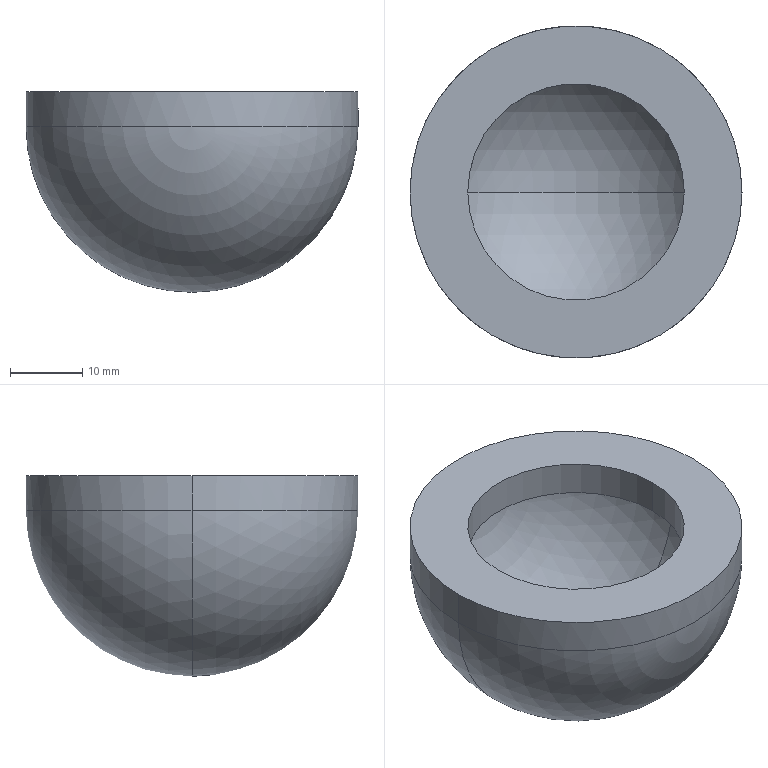Part | SolidWorks | features SavedExtBody 1 | 1 solid | 10 faces | box 46 x 46 x 27.8 mm | volume 15701 mm3 | sphere 4 | cylinder 4 | plane 2 | commonest cylinder face diameters 30 x2 46 x2
STEP:
#1=CARTESIAN_POINT('',(-19.,0.,-181.));
#2=VERTEX_POINT('',#1);
#3=CARTESIAN_POINT('',(19.,0.,-181.));
#4=VERTEX_POINT('',#3);
#5=CARTESIAN_POINT('',(0.,0.,-181.));
#6=DIRECTION('',(0.,0.,-1.));
#7=DIRECTION('',(1.,0.,0.));
#8=AXIS2_PLACEMENT_3D('',#5,#6,#7);
#9=CIRCLE('',#8,19.);
#10=EDGE_CURVE('',#2,#4,#9,.T.);
#11=ORIENTED_EDGE('',*,*,#10,.F.);
#12=CARTESIAN_POINT('',(0.,0.,-200.));
#13=VERTEX_POINT('',#12);
#14=CARTESIAN_POINT('',(0.,0.,-181.));
#15=DIRECTION('',(0.,-1.,0.));
#16=DIRECTION('',(1.,0.,0.));
#17=AXIS2_PLACEMENT_3D('',#14,#15,#16);
#18=CIRCLE('',#17,19.);
#19=EDGE_CURVE('',#2,#13,#18,.T.);
#20=ORIENTED_EDGE('',*,*,#19,.T.);
#21=CARTESIAN_POINT('',(0.,0.,-181.));
#22=DIRECTION('',(0.,1.,0.));
#23=DIRECTION('',(0.,0.,1.));
#24=AXIS2_PLACEMENT_3D('',#21,#22,#23);
#25=CIRCLE('',#24,19.);
#26=EDGE_CURVE('',#4,#13,#25,.T.);
#27=ORIENTED_EDGE('',*,*,#26,.F.);
#28=EDGE_LOOP('',(#11,#20,#27));
#29=FACE_OUTER_BOUND('',#28,.T.);
#30=CARTESIAN_POINT('',(0.,0.,-181.));
#31=DIRECTION('',(0.,-1.,0.));
#32=DIRECTION('',(1.,0.,0.));
#33=AXIS2_PLACEMENT_3D('',#30,#31,#32);
#34=SPHERICAL_SURFACE('',#33,19.);
#35=ADVANCED_FACE('',(#29),#34,.F.);
#36=CARTESIAN_POINT('',(-15.,0.,-176.2));
#37=VERTEX_POINT('',#36);
#38=CARTESIAN_POINT('',(15.,0.,-176.2));
#39=VERTEX_POINT('',#38);
#40=CARTESIAN_POINT('',(0.,0.,-176.2));
#41=DIRECTION('',(0.,0.,1.));
#42=DIRECTION('',(1.,0.,0.));
#43=AXIS2_PLACEMENT_3D('',#40,#41,#42);
#44=CIRCLE('',#43,15.);
#45=EDGE_CURVE('',#37,#39,#44,.T.);
#46=ORIENTED_EDGE('',*,*,#45,.T.);
#47=CARTESIAN_POINT('',(15.,0.,-181.));
#48=VERTEX_POINT('',#47);
#49=CARTESIAN_POINT('',(15.,0.,-176.2));
#50=DIRECTION('',(0.,0.,-1.));
#51=VECTOR('',#50,1000.);
#52=LINE('',#49,#51);
#53=EDGE_CURVE('',#39,#48,#52,.T.);
#54=ORIENTED_EDGE('',*,*,#53,.T.);
#55=CARTESIAN_POINT('',(-15.,0.,-181.));
#56=VERTEX_POINT('',#55);
#57=CARTESIAN_POINT('',(0.,0.,-181.));
#58=DIRECTION('',(0.,0.,1.));
#59=DIRECTION('',(1.,0.,0.));
#60=AXIS2_PLACEMENT_3D('',#57,#58,#59);
#61=CIRCLE('',#60,15.);
#62=EDGE_CURVE('',#56,#48,#61,.T.);
#63=ORIENTED_EDGE('',*,*,#62,.F.);
#64=CARTESIAN_POINT('',(-15.,0.,-176.2));
#65=DIRECTION('',(0.,0.,-1.));
#66=VECTOR('',#65,1000.);
#67=LINE('',#64,#66);
#68=EDGE_CURVE('',#37,#56,#67,.T.);
#69=ORIENTED_EDGE('',*,*,#68,.F.);
#70=EDGE_LOOP('',(#46,#54,#63,#69));
#71=FACE_OUTER_BOUND('',#70,.T.);
#72=CARTESIAN_POINT('',(0.,0.,-176.2));
#73=DIRECTION('',(0.,0.,-1.));
#74=DIRECTION('',(-1.,0.,0.));
#75=AXIS2_PLACEMENT_3D('',#72,#73,#74);
#76=CYLINDRICAL_SURFACE('',#75,15.);
#77=ADVANCED_FACE('',(#71),#76,.F.);
#78=CARTESIAN_POINT('',(23.,0.,-176.2));
#79=VERTEX_POINT('',#78);
#80=CARTESIAN_POINT('',(-23.,0.,-176.2));
#81=VERTEX_POINT('',#80);
#82=CARTESIAN_POINT('',(0.,0.,-176.2));
#83=DIRECTION('',(0.,0.,1.));
#84=DIRECTION('',(1.,0.,0.));
#85=AXIS2_PLACEMENT_3D('',#82,#83,#84);
#86=CIRCLE('',#85,23.);
#87=EDGE_CURVE('',#79,#81,#86,.T.);
#88=ORIENTED_EDGE('',*,*,#87,.F.);
#89=CARTESIAN_POINT('',(23.,0.,-181.));
#90=VERTEX_POINT('',#89);
#91=CARTESIAN_POINT('',(23.,0.,-176.2));
#92=DIRECTION('',(0.,0.,-1.));
#93=VECTOR('',#92,1000.);
#94=LINE('',#91,#93);
#95=EDGE_CURVE('',#79,#90,#94,.T.);
#96=ORIENTED_EDGE('',*,*,#95,.T.);
#97=CARTESIAN_POINT('',(-23.,0.,-181.));
#98=VERTEX_POINT('',#97);
#99=CARTESIAN_POINT('',(0.,0.,-181.));
#100=DIRECTION('',(0.,0.,1.));
#101=DIRECTION('',(-1.,0.,0.));
#102=AXIS2_PLACEMENT_3D('',#99,#100,#101);
#103=CIRCLE('',#102,23.);
#104=EDGE_CURVE('',#90,#98,#103,.T.);
#105=ORIENTED_EDGE('',*,*,#104,.T.);
#106=CARTESIAN_POINT('',(-23.,0.,-176.2));
#107=DIRECTION('',(0.,0.,-1.));
#108=VECTOR('',#107,1000.);
#109=LINE('',#106,#108);
#110=EDGE_CURVE('',#81,#98,#109,.T.);
#111=ORIENTED_EDGE('',*,*,#110,.F.);
#112=EDGE_LOOP('',(#88,#96,#105,#111));
#113=FACE_OUTER_BOUND('',#112,.T.);
#114=CARTESIAN_POINT('',(0.,0.,-176.2));
#115=DIRECTION('',(0.,0.,-1.));
#116=DIRECTION('',(-1.,0.,0.));
#117=AXIS2_PLACEMENT_3D('',#114,#115,#116);
#118=CYLINDRICAL_SURFACE('',#117,23.);
#119=ADVANCED_FACE('',(#113),#118,.T.);
#120=CARTESIAN_POINT('',(0.,0.,-181.));
#121=DIRECTION('',(0.,0.,1.));
#122=DIRECTION('',(-1.,0.,0.));
#123=AXIS2_PLACEMENT_3D('',#120,#121,#122);
#124=CIRCLE('',#123,23.);
#125=EDGE_CURVE('',#98,#90,#124,.T.);
#126=ORIENTED_EDGE('',*,*,#125,.F.);
#127=CARTESIAN_POINT('',(0.,0.,-204.));
#128=VERTEX_POINT('',#127);
#129=CARTESIAN_POINT('',(0.,0.,-181.));
#130=DIRECTION('',(0.,-1.,0.));
#131=DIRECTION('',(1.,0.,0.));
#132=AXIS2_PLACEMENT_3D('',#129,#130,#131);
#133=CIRCLE('',#132,23.);
#134=EDGE_CURVE('',#98,#128,#133,.T.);
#135=ORIENTED_EDGE('',*,*,#134,.T.);
#136=CARTESIAN_POINT('',(0.,0.,-181.));
#137=DIRECTION('',(0.,1.,0.));
#138=DIRECTION('',(0.,0.,1.));
#139=AXIS2_PLACEMENT_3D('',#136,#137,#138);
#140=CIRCLE('',#139,23.);
#141=EDGE_CURVE('',#90,#128,#140,.T.);
#142=ORIENTED_EDGE('',*,*,#141,.F.);
#143=EDGE_LOOP('',(#126,#135,#142));
#144=FACE_OUTER_BOUND('',#143,.T.);
#145=CARTESIAN_POINT('',(0.,0.,-181.));
#146=DIRECTION('',(0.,-1.,0.));
#147=DIRECTION('',(1.,0.,0.));
#148=AXIS2_PLACEMENT_3D('',#145,#146,#147);
#149=SPHERICAL_SURFACE('',#148,23.);
#150=ADVANCED_FACE('',(#144),#149,.T.);
#151=ORIENTED_EDGE('',*,*,#134,.F.);
#152=ORIENTED_EDGE('',*,*,#104,.F.);
#153=ORIENTED_EDGE('',*,*,#141,.T.);
#154=EDGE_LOOP('',(#151,#152,#153));
#155=FACE_OUTER_BOUND('',#154,.T.);
#156=CARTESIAN_POINT('',(0.,0.,-181.));
#157=DIRECTION('',(0.,-1.,0.));
#158=DIRECTION('',(1.,0.,0.));
#159=AXIS2_PLACEMENT_3D('',#156,#157,#158);
#160=SPHERICAL_SURFACE('',#159,23.);
#161=ADVANCED_FACE('',(#155),#160,.T.);
#162=ORIENTED_EDGE('',*,*,#62,.T.);
#163=CARTESIAN_POINT('',(0.,0.,-181.));
#164=DIRECTION('',(0.,0.,1.));
#165=DIRECTION('',(1.,0.,0.));
#166=AXIS2_PLACEMENT_3D('',#163,#164,#165);
#167=CIRCLE('',#166,15.);
#168=EDGE_CURVE('',#48,#56,#167,.T.);
#169=ORIENTED_EDGE('',*,*,#168,.T.);
#170=EDGE_LOOP('',(#162,#169));
#171=FACE_BOUND('',#170,.T.);
#172=CARTESIAN_POINT('',(0.,0.,-181.));
#173=DIRECTION('',(0.,0.,-1.));
#174=DIRECTION('',(1.,0.,0.));
#175=AXIS2_PLACEMENT_3D('',#172,#173,#174);
#176=CIRCLE('',#175,19.);
#177=EDGE_CURVE('',#4,#2,#176,.T.);
#178=ORIENTED_EDGE('',*,*,#177,.T.);
#179=ORIENTED_EDGE('',*,*,#10,.T.);
#180=EDGE_LOOP('',(#178,#179));
#181=FACE_OUTER_BOUND('',#180,.T.);
#182=CARTESIAN_POINT('',(0.,0.,-181.));
#183=DIRECTION('',(0.,0.,1.));
#184=DIRECTION('',(1.,0.,0.));
#185=AXIS2_PLACEMENT_3D('',#182,#183,#184);
#186=PLANE('',#185);
#187=ADVANCED_FACE('',(#171,#181),#186,.F.);
#188=CARTESIAN_POINT('',(0.,0.,-176.2));
#189=DIRECTION('',(0.,0.,1.));
#190=DIRECTION('',(1.,0.,0.));
#191=AXIS2_PLACEMENT_3D('',#188,#189,#190);
#192=CIRCLE('',#191,23.);
#193=EDGE_CURVE('',#81,#79,#192,.T.);
#194=ORIENTED_EDGE('',*,*,#193,.T.);
#195=ORIENTED_EDGE('',*,*,#87,.T.);
#196=EDGE_LOOP('',(#194,#195));
#197=FACE_OUTER_BOUND('',#196,.T.);
#198=ORIENTED_EDGE('',*,*,#45,.F.);
#199=CARTESIAN_POINT('',(0.,0.,-176.2));
#200=DIRECTION('',(0.,0.,1.));
#201=DIRECTION('',(1.,0.,0.));
#202=AXIS2_PLACEMENT_3D('',#199,#200,#201);
#203=CIRCLE('',#202,15.);
#204=EDGE_CURVE('',#39,#37,#203,.T.);
#205=ORIENTED_EDGE('',*,*,#204,.F.);
#206=EDGE_LOOP('',(#198,#205));
#207=FACE_BOUND('',#206,.T.);
#208=CARTESIAN_POINT('',(0.,0.,-176.2));
#209=DIRECTION('',(0.,0.,1.));
#210=DIRECTION('',(1.,0.,0.));
#211=AXIS2_PLACEMENT_3D('',#208,#209,#210);
#212=PLANE('',#211);
#213=ADVANCED_FACE('',(#197,#207),#212,.T.);
#214=ORIENTED_EDGE('',*,*,#95,.F.);
#215=ORIENTED_EDGE('',*,*,#193,.F.);
#216=ORIENTED_EDGE('',*,*,#110,.T.);
#217=ORIENTED_EDGE('',*,*,#125,.T.);
#218=EDGE_LOOP('',(#214,#215,#216,#217));
#219=FACE_OUTER_BOUND('',#218,.T.);
#220=CARTESIAN_POINT('',(0.,0.,-176.2));
#221=DIRECTION('',(0.,0.,-1.));
#222=DIRECTION('',(-1.,0.,0.));
#223=AXIS2_PLACEMENT_3D('',#220,#221,#222);
#224=CYLINDRICAL_SURFACE('',#223,23.);
#225=ADVANCED_FACE('',(#219),#224,.T.);
#226=ORIENTED_EDGE('',*,*,#53,.F.);
#227=ORIENTED_EDGE('',*,*,#204,.T.);
#228=ORIENTED_EDGE('',*,*,#68,.T.);
#229=ORIENTED_EDGE('',*,*,#168,.F.);
#230=EDGE_LOOP('',(#226,#227,#228,#229));
#231=FACE_OUTER_BOUND('',#230,.T.);
#232=CARTESIAN_POINT('',(0.,0.,-176.2));
#233=DIRECTION('',(0.,0.,-1.));
#234=DIRECTION('',(-1.,0.,0.));
#235=AXIS2_PLACEMENT_3D('',#232,#233,#234);
#236=CYLINDRICAL_SURFACE('',#235,15.);
#237=ADVANCED_FACE('',(#231),#236,.F.);
#238=ORIENTED_EDGE('',*,*,#19,.F.);
#239=ORIENTED_EDGE('',*,*,#177,.F.);
#240=ORIENTED_EDGE('',*,*,#26,.T.);
#241=EDGE_LOOP('',(#238,#239,#240));
#242=FACE_OUTER_BOUND('',#241,.T.);
#243=CARTESIAN_POINT('',(0.,0.,-181.));
#244=DIRECTION('',(0.,-1.,0.));
#245=DIRECTION('',(1.,0.,0.));
#246=AXIS2_PLACEMENT_3D('',#243,#244,#245);
#247=SPHERICAL_SURFACE('',#246,19.);
#248=ADVANCED_FACE('',(#242),#247,.F.);
#249=CLOSED_SHELL('',(#35,#77,#119,#150,#161,#187,#213,#225,#237,#248));
#250=MANIFOLD_SOLID_BREP('',#249);
#251=CARTESIAN_POINT('',(0.,0.,0.));
#252=DIRECTION('',(0.,0.,1.));
#253=DIRECTION('',(1.,0.,0.));
#254=AXIS2_PLACEMENT_3D('',#251,#252,#253);
#255=(LENGTH_UNIT()NAMED_UNIT(*)SI_UNIT(.MILLI.,.METRE.));
#256=UNCERTAINTY_MEASURE_WITH_UNIT(LENGTH_MEASURE(0.00001),#255,'','');
#257=(NAMED_UNIT(*)PLANE_ANGLE_UNIT()SI_UNIT($,.RADIAN.));
#258=(NAMED_UNIT(*)SI_UNIT($,.STERADIAN.)SOLID_ANGLE_UNIT());
#259=(GEOMETRIC_REPRESENTATION_CONTEXT(3)GLOBAL_UNCERTAINTY_ASSIGNED_CONTEXT((#256))GLOBAL_UNIT_ASSIGNED_CONTEXT((#255,#257,#258))REPRESENTATION_CONTEXT('',''));
#260=ADVANCED_BREP_SHAPE_REPRESENTATION('',(#250,#254),#259);